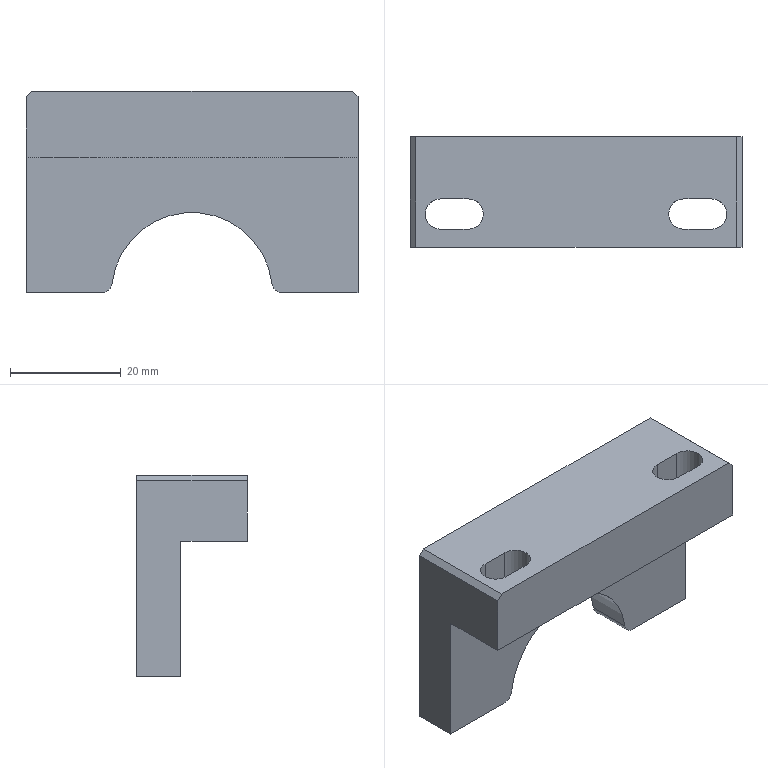CAM job | NX | 3+2 milling | part box 60 x 20 x 36.5 mm | stock box 65 x 25 x 41.5 mm
Tools:
number,name,description,diameter,corner_radius,flute_length,length,flutes
4,D4,平底铣刀-粗,4.0,0.0,25.0,75.0,2
9,D10,平底铣刀-粗,10.0,0.0,35.0,75.0,2
11,D4-J,平底铣刀-精,4.0,0.0,50.0,75.0,2
7,D6-J,平底铣刀-精,6.0,0.0,25.0,75.0,2
1,D80R0.8飞刀,圆鼻刀-粗,80.0,0.8,50.0,75.0,2
1,D80R0.8飞刀-J,圆鼻刀-精,80.0,0.8,50.0,75.0,2
2,D6倒角刀,倒角刀,6.0,0.0,3.0,25.0,2
Operations:
program,operation,operation_type,tool,method,geometry_group,spindle_rpm,surface_speed,feed_per_tooth,feed_cut,feed_plunge,cut_length_mm,path_length_mm,cut_time_min,machine_time_min
C,底壁铣螺旋开粗-小_COPY,VolumeBased25DMillingOperation,D4,分层开粗-切深K-步距G,W-C,8000.0,100.528,0.125,2000.0,100.0,1244.466,1511.32,0.6222,0.6489
C,底壁铣螺旋精光-小_COPY,VolumeBased25DMillingOperation,D4-J,螺旋精光-切深K-步距G,W-C,8000.0,100.528,0.05,800.0,100.0,259.174,520.688,0.324,0.3501
C,C0.3封闭铣廓倒角6X45L_COPY,PlanarMilling,D6倒角刀,爬面_倒角-切深0-步距G,W-C,7000.0,131.0,0.1071,1500.0,100.0,72.228,311.079,0.0482,0.072
B,底壁铣飞面一刀开粗_COPY,VolumeBased25DMillingOperation,D80R0.8飞刀,分层开粗-切深K-步距G,W-B,2800.0,703.696,0.5357,3000.0,100.0,1513.746,3385.967,0.5046,0.6918
B,底壁铣飞面一刀精光_COPY,VolumeBased25DMillingOperation,D80R0.8飞刀-J,侧刃精光-切深K-步距G,W-B,4000.0,1005.28,0.125,1000.0,100.0,167.998,263.998,0.168,0.1776
B,底壁铣分层开粗-中_COPY,VolumeBased25DMillingOperation,D10,分层开粗-切深K-步距G,W-B,8000.0,251.32,0.25,4000.0,100.0,8085.08,8138.342,2.021,2.027
B,平面去毛刺6X45L_COPY,SurfaceContour,D6倒角刀,爬面_倒角-切深0-步距G,W-B,6500.0,122.519,0.1154,1500.0,100.0,296.847,451.629,0.1979,0.2134
B,底壁铣精光底面-中_COPY,VolumeBased25DMillingOperation,D6-J,精光步距切深关,W-B,8000.0,150.792,0.0625,1000.0,100.0,455.388,505.388,0.4554,0.4604
B,底壁铣精光侧面-中-选底面_COPY,VolumeBased25DMillingOperation,D6-J,侧刃精光-切深K-步距G,W-B,8000.0,150.792,0.0625,1000.0,100.0,72.169,123.169,0.0722,0.0773
A,顶面,FaceMilling,D80R0.8飞刀,侧刃精光-切深K-步距G,W-A,4500.0,1385.0,0.1667,1500.0,100.0,154.0,250.0,0.1027,0.1123
A,动态开粗D10_COPY,CavityMilling,D10,动态开粗-切深K-步距K,W-A,8000.0,251.32,0.25,4000.0,100.0,1749.336,1885.336,0.4373,0.4509
A,仅选体,SurfaceContour,D6倒角刀,METHOD,W-A,8000.0,150.796,0.1875,3000.0,100.0,224.263,320.064,0.0748,0.0843
A,外形半精_2,VolumeBased25DMillingOperation,D6-J,METHOD,W-A,9000.0,169.646,0.0667,1200.0,100.0,461.441,721.961,0.3845,0.4106